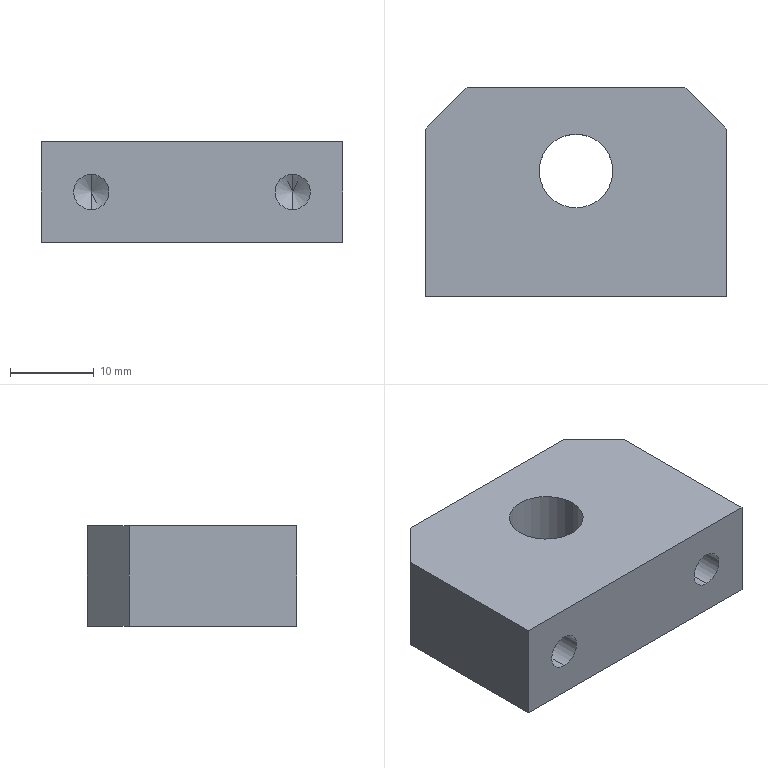Part | STEP file | 2037 Bag feed mounting plate 3 | 1 solid | 18 faces | box 36 x 25 x 12 mm | volume 9371 mm3 | plane 8 | cylinder 6 | cone 4 | commonest cylinder face diameters 4.2 x4 8.8 x2
STEP:
#1=CARTESIAN_POINT('',(0.,0.,0.));
#2=DIRECTION('',(0.,0.,1.));
#3=DIRECTION('',(1.,0.,0.));
#4=AXIS2_PLACEMENT_3D('',#1,#2,#3);
#5=CARTESIAN_POINT('',(12.,1.5,3.9));
#6=VERTEX_POINT('',#5);
#7=CARTESIAN_POINT('',(12.,-12.5,3.9));
#8=VERTEX_POINT('',#7);
#9=CARTESIAN_POINT('',(12.,-12.5,3.9));
#10=DIRECTION('',(0.,-1.,0.));
#11=VECTOR('',#10,1.);
#12=LINE('',#9,#11);
#13=CARTESIAN_POINT('',(12.,-12.5,6.));
#14=DIRECTION('',(0.,-1.,0.));
#15=DIRECTION('',(0.,0.,-1.));
#16=AXIS2_PLACEMENT_3D('',#13,#14,#15);
#17=CYLINDRICAL_SURFACE('',#16,2.1);
#18=CARTESIAN_POINT('',(6.283,0.));
#19=DIRECTION('',(0.,1.));
#20=VECTOR('',#19,1.);
#21=LINE('',#18,#20);
#22=(GEOMETRIC_REPRESENTATION_CONTEXT(2)PARAMETRIC_REPRESENTATION_CONTEXT()REPRESENTATION_CONTEXT('',''));
#23=DEFINITIONAL_REPRESENTATION('',(#21),#22);
#24=PCURVE('',#17,#23);
#25=CARTESIAN_POINT('',(12.,-12.5,6.));
#26=DIRECTION('',(0.,-1.,0.));
#27=DIRECTION('',(0.,0.,-1.));
#28=AXIS2_PLACEMENT_3D('',#25,#26,#27);
#29=CYLINDRICAL_SURFACE('',#28,2.1);
#30=CARTESIAN_POINT('',(0.,0.));
#31=DIRECTION('',(0.,1.));
#32=VECTOR('',#31,1.);
#33=LINE('',#30,#32);
#34=(GEOMETRIC_REPRESENTATION_CONTEXT(2)PARAMETRIC_REPRESENTATION_CONTEXT()REPRESENTATION_CONTEXT('',''));
#35=DEFINITIONAL_REPRESENTATION('',(#33),#34);
#36=PCURVE('',#29,#35);
#37=SURFACE_CURVE('',#12,(#24,#36),.PCURVE_S1.);
#38=EDGE_CURVE('',#6,#8,#37,.T.);
#39=ORIENTED_EDGE('',*,*,#38,.T.);
#40=CARTESIAN_POINT('',(12.,-12.5,8.1));
#41=VERTEX_POINT('',#40);
#42=CARTESIAN_POINT('',(12.,-12.5,6.));
#43=DIRECTION('',(0.,-1.,0.));
#44=DIRECTION('',(0.,0.,-1.));
#45=AXIS2_PLACEMENT_3D('',#42,#43,#44);
#46=CIRCLE('',#45,2.1);
#47=CARTESIAN_POINT('',(0.,0.));
#48=DIRECTION('',(1.,0.));
#49=VECTOR('',#48,1.);
#50=LINE('',#47,#49);
#51=(GEOMETRIC_REPRESENTATION_CONTEXT(2)PARAMETRIC_REPRESENTATION_CONTEXT()REPRESENTATION_CONTEXT('',''));
#52=DEFINITIONAL_REPRESENTATION('',(#50),#51);
#53=PCURVE('',#17,#52);
#54=CARTESIAN_POINT('',(-18.,-12.5,12.));
#55=DIRECTION('',(0.,1.,0.));
#56=DIRECTION('',(0.,0.,1.));
#57=AXIS2_PLACEMENT_3D('',#54,#55,#56);
#58=PLANE('',#57);
#59=CARTESIAN_POINT('',(-8.1,30.));
#60=CARTESIAN_POINT('',(-8.1,33.637));
#61=CARTESIAN_POINT('',(-4.95,31.819));
#62=CARTESIAN_POINT('',(-1.8,30.));
#63=CARTESIAN_POINT('',(-4.95,28.181));
#64=CARTESIAN_POINT('',(-8.1,26.363));
#65=CARTESIAN_POINT('',(-8.1,30.));
#66=(BOUNDED_CURVE()B_SPLINE_CURVE(2,(#59,#60,#61,#62,#63,#64,#65),.UNSPECIFIED.,.T.,.F.)B_SPLINE_CURVE_WITH_KNOTS((1,2,2,2,2,1),(-2.094,0.,2.094,4.189,6.283,8.378),.UNSPECIFIED.)CURVE()GEOMETRIC_REPRESENTATION_ITEM()RATIONAL_B_SPLINE_CURVE((1.,0.5,1.,0.5,1.,0.5,1.))REPRESENTATION_ITEM(''));
#67=(GEOMETRIC_REPRESENTATION_CONTEXT(2)PARAMETRIC_REPRESENTATION_CONTEXT()REPRESENTATION_CONTEXT('',''));
#68=DEFINITIONAL_REPRESENTATION('',(#66),#67);
#69=PCURVE('',#58,#68);
#70=SURFACE_CURVE('',#46,(#53,#69),.PCURVE_S1.);
#71=EDGE_CURVE('',#41,#8,#70,.T.);
#72=ORIENTED_EDGE('',*,*,#71,.F.);
#73=CARTESIAN_POINT('',(12.,1.5,8.1));
#74=VERTEX_POINT('',#73);
#75=CARTESIAN_POINT('',(12.,-12.5,8.1));
#76=DIRECTION('',(0.,-1.,0.));
#77=VECTOR('',#76,1.);
#78=LINE('',#75,#77);
#79=CARTESIAN_POINT('',(3.142,0.));
#80=DIRECTION('',(0.,1.));
#81=VECTOR('',#80,1.);
#82=LINE('',#79,#81);
#83=(GEOMETRIC_REPRESENTATION_CONTEXT(2)PARAMETRIC_REPRESENTATION_CONTEXT()REPRESENTATION_CONTEXT('',''));
#84=DEFINITIONAL_REPRESENTATION('',(#82),#83);
#85=PCURVE('',#17,#84);
#86=CARTESIAN_POINT('',(3.142,0.));
#87=DIRECTION('',(0.,1.));
#88=VECTOR('',#87,1.);
#89=LINE('',#86,#88);
#90=(GEOMETRIC_REPRESENTATION_CONTEXT(2)PARAMETRIC_REPRESENTATION_CONTEXT()REPRESENTATION_CONTEXT('',''));
#91=DEFINITIONAL_REPRESENTATION('',(#89),#90);
#92=PCURVE('',#29,#91);
#93=SURFACE_CURVE('',#78,(#85,#92),.PCURVE_S1.);
#94=EDGE_CURVE('',#74,#41,#93,.T.);
#95=ORIENTED_EDGE('',*,*,#94,.F.);
#96=CARTESIAN_POINT('',(12.,1.5,6.));
#97=DIRECTION('',(0.,-1.,0.));
#98=DIRECTION('',(0.,0.,-1.));
#99=AXIS2_PLACEMENT_3D('',#96,#97,#98);
#100=CIRCLE('',#99,2.1);
#101=CARTESIAN_POINT('',(0.,-14.));
#102=DIRECTION('',(1.,0.));
#103=VECTOR('',#102,1.);
#104=LINE('',#101,#103);
#105=(GEOMETRIC_REPRESENTATION_CONTEXT(2)PARAMETRIC_REPRESENTATION_CONTEXT()REPRESENTATION_CONTEXT('',''));
#106=DEFINITIONAL_REPRESENTATION('',(#104),#105);
#107=PCURVE('',#17,#106);
#108=CARTESIAN_POINT('',(12.,1.5,6.));
#109=DIRECTION('',(0.,-1.,0.));
#110=DIRECTION('',(0.,0.,-1.));
#111=AXIS2_PLACEMENT_3D('',#108,#109,#110);
#112=CONICAL_SURFACE('',#111,2.1,1.03);
#113=CARTESIAN_POINT('',(0.,0.));
#114=DIRECTION('',(1.,0.));
#115=VECTOR('',#114,1.);
#116=LINE('',#113,#115);
#117=(GEOMETRIC_REPRESENTATION_CONTEXT(2)PARAMETRIC_REPRESENTATION_CONTEXT()REPRESENTATION_CONTEXT('',''));
#118=DEFINITIONAL_REPRESENTATION('',(#116),#117);
#119=PCURVE('',#112,#118);
#120=SURFACE_CURVE('',#100,(#107,#119),.PCURVE_S1.);
#121=EDGE_CURVE('',#74,#6,#120,.T.);
#122=ORIENTED_EDGE('',*,*,#121,.T.);
#123=EDGE_LOOP('',(#39,#72,#95,#122));
#124=FACE_BOUND('',#123,.F.);
#125=ADVANCED_FACE('',(#124),#17,.F.);
#126=ORIENTED_EDGE('',*,*,#121,.F.);
#127=CARTESIAN_POINT('',(12.,2.762,6.));
#128=VERTEX_POINT('',#127);
#129=CARTESIAN_POINT('',(12.,1.5,8.1));
#130=DIRECTION('',(0.,-0.515,0.8572));
#131=VECTOR('',#130,1.);
#132=LINE('',#129,#131);
#133=CARTESIAN_POINT('',(3.142,0.));
#134=DIRECTION('',(0.,1.));
#135=VECTOR('',#134,1.);
#136=LINE('',#133,#135);
#137=(GEOMETRIC_REPRESENTATION_CONTEXT(2)PARAMETRIC_REPRESENTATION_CONTEXT()REPRESENTATION_CONTEXT('',''));
#138=DEFINITIONAL_REPRESENTATION('',(#136),#137);
#139=PCURVE('',#112,#138);
#140=CARTESIAN_POINT('',(12.,1.5,6.));
#141=DIRECTION('',(0.,-1.,0.));
#142=DIRECTION('',(0.,0.,-1.));
#143=AXIS2_PLACEMENT_3D('',#140,#141,#142);
#144=CONICAL_SURFACE('',#143,2.1,1.03);
#145=CARTESIAN_POINT('',(3.142,0.));
#146=DIRECTION('',(0.,1.));
#147=VECTOR('',#146,1.);
#148=LINE('',#145,#147);
#149=(GEOMETRIC_REPRESENTATION_CONTEXT(2)PARAMETRIC_REPRESENTATION_CONTEXT()REPRESENTATION_CONTEXT('',''));
#150=DEFINITIONAL_REPRESENTATION('',(#148),#149);
#151=PCURVE('',#144,#150);
#152=SURFACE_CURVE('',#132,(#139,#151),.PCURVE_S1.);
#153=EDGE_CURVE('',#128,#74,#152,.T.);
#154=ORIENTED_EDGE('',*,*,#153,.F.);
#155=CARTESIAN_POINT('',(12.,1.5,3.9));
#156=DIRECTION('',(0.,-0.515,-0.8572));
#157=VECTOR('',#156,1.);
#158=LINE('',#155,#157);
#159=CARTESIAN_POINT('',(6.283,0.));
#160=DIRECTION('',(0.,1.));
#161=VECTOR('',#160,1.);
#162=LINE('',#159,#161);
#163=(GEOMETRIC_REPRESENTATION_CONTEXT(2)PARAMETRIC_REPRESENTATION_CONTEXT()REPRESENTATION_CONTEXT('',''));
#164=DEFINITIONAL_REPRESENTATION('',(#162),#163);
#165=PCURVE('',#112,#164);
#166=CARTESIAN_POINT('',(0.,0.));
#167=DIRECTION('',(0.,1.));
#168=VECTOR('',#167,1.);
#169=LINE('',#166,#168);
#170=(GEOMETRIC_REPRESENTATION_CONTEXT(2)PARAMETRIC_REPRESENTATION_CONTEXT()REPRESENTATION_CONTEXT('',''));
#171=DEFINITIONAL_REPRESENTATION('',(#169),#170);
#172=PCURVE('',#144,#171);
#173=SURFACE_CURVE('',#158,(#165,#172),.PCURVE_S1.);
#174=EDGE_CURVE('',#128,#6,#173,.T.);
#175=ORIENTED_EDGE('',*,*,#174,.T.);
#176=EDGE_LOOP('',(#126,#154,#175));
#177=FACE_BOUND('',#176,.F.);
#178=ADVANCED_FACE('',(#177),#112,.F.);
#179=CARTESIAN_POINT('',(-12.,1.5,3.9));
#180=VERTEX_POINT('',#179);
#181=CARTESIAN_POINT('',(-12.,-12.5,3.9));
#182=VERTEX_POINT('',#181);
#183=CARTESIAN_POINT('',(-12.,-12.5,3.9));
#184=DIRECTION('',(0.,-1.,0.));
#185=VECTOR('',#184,1.);
#186=LINE('',#183,#185);
#187=CARTESIAN_POINT('',(-12.,-12.5,6.));
#188=DIRECTION('',(0.,-1.,0.));
#189=DIRECTION('',(0.,0.,-1.));
#190=AXIS2_PLACEMENT_3D('',#187,#188,#189);
#191=CYLINDRICAL_SURFACE('',#190,2.1);
#192=CARTESIAN_POINT('',(6.283,0.));
#193=DIRECTION('',(0.,1.));
#194=VECTOR('',#193,1.);
#195=LINE('',#192,#194);
#196=(GEOMETRIC_REPRESENTATION_CONTEXT(2)PARAMETRIC_REPRESENTATION_CONTEXT()REPRESENTATION_CONTEXT('',''));
#197=DEFINITIONAL_REPRESENTATION('',(#195),#196);
#198=PCURVE('',#191,#197);
#199=CARTESIAN_POINT('',(-12.,-12.5,6.));
#200=DIRECTION('',(0.,-1.,0.));
#201=DIRECTION('',(0.,0.,-1.));
#202=AXIS2_PLACEMENT_3D('',#199,#200,#201);
#203=CYLINDRICAL_SURFACE('',#202,2.1);
#204=CARTESIAN_POINT('',(0.,0.));
#205=DIRECTION('',(0.,1.));
#206=VECTOR('',#205,1.);
#207=LINE('',#204,#206);
#208=(GEOMETRIC_REPRESENTATION_CONTEXT(2)PARAMETRIC_REPRESENTATION_CONTEXT()REPRESENTATION_CONTEXT('',''));
#209=DEFINITIONAL_REPRESENTATION('',(#207),#208);
#210=PCURVE('',#203,#209);
#211=SURFACE_CURVE('',#186,(#198,#210),.PCURVE_S1.);
#212=EDGE_CURVE('',#180,#182,#211,.T.);
#213=ORIENTED_EDGE('',*,*,#212,.T.);
#214=CARTESIAN_POINT('',(-12.,-12.5,8.1));
#215=VERTEX_POINT('',#214);
#216=CARTESIAN_POINT('',(-12.,-12.5,6.));
#217=DIRECTION('',(0.,-1.,0.));
#218=DIRECTION('',(0.,0.,-1.));
#219=AXIS2_PLACEMENT_3D('',#216,#217,#218);
#220=CIRCLE('',#219,2.1);
#221=CARTESIAN_POINT('',(0.,0.));
#222=DIRECTION('',(1.,0.));
#223=VECTOR('',#222,1.);
#224=LINE('',#221,#223);
#225=(GEOMETRIC_REPRESENTATION_CONTEXT(2)PARAMETRIC_REPRESENTATION_CONTEXT()REPRESENTATION_CONTEXT('',''));
#226=DEFINITIONAL_REPRESENTATION('',(#224),#225);
#227=PCURVE('',#191,#226);
#228=CARTESIAN_POINT('',(-8.1,6.));
#229=CARTESIAN_POINT('',(-8.1,9.637));
#230=CARTESIAN_POINT('',(-4.95,7.819));
#231=CARTESIAN_POINT('',(-1.8,6.));
#232=CARTESIAN_POINT('',(-4.95,4.181));
#233=CARTESIAN_POINT('',(-8.1,2.363));
#234=CARTESIAN_POINT('',(-8.1,6.));
#235=(BOUNDED_CURVE()B_SPLINE_CURVE(2,(#228,#229,#230,#231,#232,#233,#234),.UNSPECIFIED.,.T.,.F.)B_SPLINE_CURVE_WITH_KNOTS((1,2,2,2,2,1),(-2.094,0.,2.094,4.189,6.283,8.378),.UNSPECIFIED.)CURVE()GEOMETRIC_REPRESENTATION_ITEM()RATIONAL_B_SPLINE_CURVE((1.,0.5,1.,0.5,1.,0.5,1.))REPRESENTATION_ITEM(''));
#236=(GEOMETRIC_REPRESENTATION_CONTEXT(2)PARAMETRIC_REPRESENTATION_CONTEXT()REPRESENTATION_CONTEXT('',''));
#237=DEFINITIONAL_REPRESENTATION('',(#235),#236);
#238=PCURVE('',#58,#237);
#239=SURFACE_CURVE('',#220,(#227,#238),.PCURVE_S1.);
#240=EDGE_CURVE('',#215,#182,#239,.T.);
#241=ORIENTED_EDGE('',*,*,#240,.F.);
#242=CARTESIAN_POINT('',(-12.,1.5,8.1));
#243=VERTEX_POINT('',#242);
#244=CARTESIAN_POINT('',(-12.,-12.5,8.1));
#245=DIRECTION('',(0.,-1.,0.));
#246=VECTOR('',#245,1.);
#247=LINE('',#244,#246);
#248=CARTESIAN_POINT('',(3.142,0.));
#249=DIRECTION('',(0.,1.));
#250=VECTOR('',#249,1.);
#251=LINE('',#248,#250);
#252=(GEOMETRIC_REPRESENTATION_CONTEXT(2)PARAMETRIC_REPRESENTATION_CONTEXT()REPRESENTATION_CONTEXT('',''));
#253=DEFINITIONAL_REPRESENTATION('',(#251),#252);
#254=PCURVE('',#191,#253);
#255=CARTESIAN_POINT('',(3.142,0.));
#256=DIRECTION('',(0.,1.));
#257=VECTOR('',#256,1.);
#258=LINE('',#255,#257);
#259=(GEOMETRIC_REPRESENTATION_CONTEXT(2)PARAMETRIC_REPRESENTATION_CONTEXT()REPRESENTATION_CONTEXT('',''));
#260=DEFINITIONAL_REPRESENTATION('',(#258),#259);
#261=PCURVE('',#203,#260);
#262=SURFACE_CURVE('',#247,(#254,#261),.PCURVE_S1.);
#263=EDGE_CURVE('',#243,#215,#262,.T.);
#264=ORIENTED_EDGE('',*,*,#263,.F.);
#265=CARTESIAN_POINT('',(-12.,1.5,6.));
#266=DIRECTION('',(0.,-1.,0.));
#267=DIRECTION('',(0.,0.,-1.));
#268=AXIS2_PLACEMENT_3D('',#265,#266,#267);
#269=CIRCLE('',#268,2.1);
#270=CARTESIAN_POINT('',(0.,-14.));
#271=DIRECTION('',(1.,0.));
#272=VECTOR('',#271,1.);
#273=LINE('',#270,#272);
#274=(GEOMETRIC_REPRESENTATION_CONTEXT(2)PARAMETRIC_REPRESENTATION_CONTEXT()REPRESENTATION_CONTEXT('',''));
#275=DEFINITIONAL_REPRESENTATION('',(#273),#274);
#276=PCURVE('',#191,#275);
#277=CARTESIAN_POINT('',(-12.,1.5,6.));
#278=DIRECTION('',(0.,-1.,0.));
#279=DIRECTION('',(0.,0.,-1.));
#280=AXIS2_PLACEMENT_3D('',#277,#278,#279);
#281=CONICAL_SURFACE('',#280,2.1,1.03);
#282=CARTESIAN_POINT('',(0.,0.));
#283=DIRECTION('',(1.,0.));
#284=VECTOR('',#283,1.);
#285=LINE('',#282,#284);
#286=(GEOMETRIC_REPRESENTATION_CONTEXT(2)PARAMETRIC_REPRESENTATION_CONTEXT()REPRESENTATION_CONTEXT('',''));
#287=DEFINITIONAL_REPRESENTATION('',(#285),#286);
#288=PCURVE('',#281,#287);
#289=SURFACE_CURVE('',#269,(#276,#288),.PCURVE_S1.);
#290=EDGE_CURVE('',#243,#180,#289,.T.);
#291=ORIENTED_EDGE('',*,*,#290,.T.);
#292=EDGE_LOOP('',(#213,#241,#264,#291));
#293=FACE_BOUND('',#292,.F.);
#294=ADVANCED_FACE('',(#293),#191,.F.);
#295=ORIENTED_EDGE('',*,*,#290,.F.);
#296=CARTESIAN_POINT('',(-12.,2.762,6.));
#297=VERTEX_POINT('',#296);
#298=CARTESIAN_POINT('',(-12.,1.5,8.1));
#299=DIRECTION('',(0.,-0.515,0.8572));
#300=VECTOR('',#299,1.);
#301=LINE('',#298,#300);
#302=CARTESIAN_POINT('',(3.142,0.));
#303=DIRECTION('',(0.,1.));
#304=VECTOR('',#303,1.);
#305=LINE('',#302,#304);
#306=(GEOMETRIC_REPRESENTATION_CONTEXT(2)PARAMETRIC_REPRESENTATION_CONTEXT()REPRESENTATION_CONTEXT('',''));
#307=DEFINITIONAL_REPRESENTATION('',(#305),#306);
#308=PCURVE('',#281,#307);
#309=CARTESIAN_POINT('',(-12.,1.5,6.));
#310=DIRECTION('',(0.,-1.,0.));
#311=DIRECTION('',(0.,0.,-1.));
#312=AXIS2_PLACEMENT_3D('',#309,#310,#311);
#313=CONICAL_SURFACE('',#312,2.1,1.03);
#314=CARTESIAN_POINT('',(3.142,0.));
#315=DIRECTION('',(0.,1.));
#316=VECTOR('',#315,1.);
#317=LINE('',#314,#316);
#318=(GEOMETRIC_REPRESENTATION_CONTEXT(2)PARAMETRIC_REPRESENTATION_CONTEXT()REPRESENTATION_CONTEXT('',''));
#319=DEFINITIONAL_REPRESENTATION('',(#317),#318);
#320=PCURVE('',#313,#319);
#321=SURFACE_CURVE('',#301,(#308,#320),.PCURVE_S1.);
#322=EDGE_CURVE('',#297,#243,#321,.T.);
#323=ORIENTED_EDGE('',*,*,#322,.F.);
#324=CARTESIAN_POINT('',(-12.,1.5,3.9));
#325=DIRECTION('',(0.,-0.515,-0.8572));
#326=VECTOR('',#325,1.);
#327=LINE('',#324,#326);
#328=CARTESIAN_POINT('',(6.283,0.));
#329=DIRECTION('',(0.,1.));
#330=VECTOR('',#329,1.);
#331=LINE('',#328,#330);
#332=(GEOMETRIC_REPRESENTATION_CONTEXT(2)PARAMETRIC_REPRESENTATION_CONTEXT()REPRESENTATION_CONTEXT('',''));
#333=DEFINITIONAL_REPRESENTATION('',(#331),#332);
#334=PCURVE('',#281,#333);
#335=CARTESIAN_POINT('',(0.,0.));
#336=DIRECTION('',(0.,1.));
#337=VECTOR('',#336,1.);
#338=LINE('',#335,#337);
#339=(GEOMETRIC_REPRESENTATION_CONTEXT(2)PARAMETRIC_REPRESENTATION_CONTEXT()REPRESENTATION_CONTEXT('',''));
#340=DEFINITIONAL_REPRESENTATION('',(#338),#339);
#341=PCURVE('',#313,#340);
#342=SURFACE_CURVE('',#327,(#334,#341),.PCURVE_S1.);
#343=EDGE_CURVE('',#297,#180,#342,.T.);
#344=ORIENTED_EDGE('',*,*,#343,.T.);
#345=EDGE_LOOP('',(#295,#323,#344));
#346=FACE_BOUND('',#345,.F.);
#347=ADVANCED_FACE('',(#346),#281,.F.);
#348=CARTESIAN_POINT('',(4.4,2.5,0.));
#349=VERTEX_POINT('',#348);
#350=CARTESIAN_POINT('',(4.4,2.5,12.));
#351=VERTEX_POINT('',#350);
#352=CARTESIAN_POINT('',(4.4,2.5,12.));
#353=DIRECTION('',(0.,0.,1.));
#354=VECTOR('',#353,1.);
#355=LINE('',#352,#354);
#356=CARTESIAN_POINT('',(0.,2.5,12.));
#357=DIRECTION('',(0.,0.,1.));
#358=DIRECTION('',(1.,0.,0.));
#359=AXIS2_PLACEMENT_3D('',#356,#357,#358);
#360=CYLINDRICAL_SURFACE('',#359,4.4);
#361=CARTESIAN_POINT('',(6.283,0.));
#362=DIRECTION('',(0.,1.));
#363=VECTOR('',#362,1.);
#364=LINE('',#361,#363);
#365=(GEOMETRIC_REPRESENTATION_CONTEXT(2)PARAMETRIC_REPRESENTATION_CONTEXT()REPRESENTATION_CONTEXT('',''));
#366=DEFINITIONAL_REPRESENTATION('',(#364),#365);
#367=PCURVE('',#360,#366);
#368=CARTESIAN_POINT('',(0.,2.5,12.));
#369=DIRECTION('',(0.,0.,1.));
#370=DIRECTION('',(1.,0.,0.));
#371=AXIS2_PLACEMENT_3D('',#368,#369,#370);
#372=CYLINDRICAL_SURFACE('',#371,4.4);
#373=CARTESIAN_POINT('',(0.,0.));
#374=DIRECTION('',(0.,1.));
#375=VECTOR('',#374,1.);
#376=LINE('',#373,#375);
#377=(GEOMETRIC_REPRESENTATION_CONTEXT(2)PARAMETRIC_REPRESENTATION_CONTEXT()REPRESENTATION_CONTEXT('',''));
#378=DEFINITIONAL_REPRESENTATION('',(#376),#377);
#379=PCURVE('',#372,#378);
#380=SURFACE_CURVE('',#355,(#367,#379),.PCURVE_S1.);
#381=EDGE_CURVE('',#349,#351,#380,.T.);
#382=ORIENTED_EDGE('',*,*,#381,.T.);
#383=CARTESIAN_POINT('',(-4.4,2.5,12.));
#384=VERTEX_POINT('',#383);
#385=CARTESIAN_POINT('',(0.,2.5,12.));
#386=DIRECTION('',(0.,0.,1.));
#387=DIRECTION('',(1.,0.,0.));
#388=AXIS2_PLACEMENT_3D('',#385,#386,#387);
#389=CIRCLE('',#388,4.4);
#390=CARTESIAN_POINT('',(0.,0.));
#391=DIRECTION('',(1.,0.));
#392=VECTOR('',#391,1.);
#393=LINE('',#390,#392);
#394=(GEOMETRIC_REPRESENTATION_CONTEXT(2)PARAMETRIC_REPRESENTATION_CONTEXT()REPRESENTATION_CONTEXT('',''));
#395=DEFINITIONAL_REPRESENTATION('',(#393),#394);
#396=PCURVE('',#360,#395);
#397=CARTESIAN_POINT('',(0.,0.,12.));
#398=DIRECTION('',(0.,0.,-1.));
#399=DIRECTION('',(-1.,0.,0.));
#400=AXIS2_PLACEMENT_3D('',#397,#398,#399);
#401=PLANE('',#400);
#402=CARTESIAN_POINT('',(-4.4,2.5));
#403=CARTESIAN_POINT('',(-4.4,10.121));
#404=CARTESIAN_POINT('',(2.2,6.311));
#405=CARTESIAN_POINT('',(8.8,2.5));
#406=CARTESIAN_POINT('',(2.2,-1.311));
#407=CARTESIAN_POINT('',(-4.4,-5.121));
#408=CARTESIAN_POINT('',(-4.4,2.5));
#409=(BOUNDED_CURVE()B_SPLINE_CURVE(2,(#402,#403,#404,#405,#406,#407,#408),.UNSPECIFIED.,.T.,.F.)B_SPLINE_CURVE_WITH_KNOTS((1,2,2,2,2,1),(-2.094,0.,2.094,4.189,6.283,8.378),.UNSPECIFIED.)CURVE()GEOMETRIC_REPRESENTATION_ITEM()RATIONAL_B_SPLINE_CURVE((1.,0.5,1.,0.5,1.,0.5,1.))REPRESENTATION_ITEM(''));
#410=(GEOMETRIC_REPRESENTATION_CONTEXT(2)PARAMETRIC_REPRESENTATION_CONTEXT()REPRESENTATION_CONTEXT('',''));
#411=DEFINITIONAL_REPRESENTATION('',(#409),#410);
#412=PCURVE('',#401,#411);
#413=SURFACE_CURVE('',#389,(#396,#412),.PCURVE_S1.);
#414=EDGE_CURVE('',#384,#351,#413,.T.);
#415=ORIENTED_EDGE('',*,*,#414,.F.);
#416=CARTESIAN_POINT('',(-4.4,2.5,0.));
#417=VERTEX_POINT('',#416);
#418=CARTESIAN_POINT('',(-4.4,2.5,12.));
#419=DIRECTION('',(0.,0.,1.));
#420=VECTOR('',#419,1.);
#421=LINE('',#418,#420);
#422=CARTESIAN_POINT('',(3.142,0.));
#423=DIRECTION('',(0.,1.));
#424=VECTOR('',#423,1.);
#425=LINE('',#422,#424);
#426=(GEOMETRIC_REPRESENTATION_CONTEXT(2)PARAMETRIC_REPRESENTATION_CONTEXT()REPRESENTATION_CONTEXT('',''));
#427=DEFINITIONAL_REPRESENTATION('',(#425),#426);
#428=PCURVE('',#360,#427);
#429=CARTESIAN_POINT('',(3.142,0.));
#430=DIRECTION('',(0.,1.));
#431=VECTOR('',#430,1.);
#432=LINE('',#429,#431);
#433=(GEOMETRIC_REPRESENTATION_CONTEXT(2)PARAMETRIC_REPRESENTATION_CONTEXT()REPRESENTATION_CONTEXT('',''));
#434=DEFINITIONAL_REPRESENTATION('',(#432),#433);
#435=PCURVE('',#372,#434);
#436=SURFACE_CURVE('',#421,(#428,#435),.PCURVE_S1.);
#437=EDGE_CURVE('',#417,#384,#436,.T.);
#438=ORIENTED_EDGE('',*,*,#437,.F.);
#439=CARTESIAN_POINT('',(0.,2.5,0.));
#440=DIRECTION('',(0.,0.,1.));
#441=DIRECTION('',(1.,0.,0.));
#442=AXIS2_PLACEMENT_3D('',#439,#440,#441);
#443=CIRCLE('',#442,4.4);
#444=CARTESIAN_POINT('',(0.,-12.));
#445=DIRECTION('',(1.,0.));
#446=VECTOR('',#445,1.);
#447=LINE('',#444,#446);
#448=(GEOMETRIC_REPRESENTATION_CONTEXT(2)PARAMETRIC_REPRESENTATION_CONTEXT()REPRESENTATION_CONTEXT('',''));
#449=DEFINITIONAL_REPRESENTATION('',(#447),#448);
#450=PCURVE('',#360,#449);
#451=CARTESIAN_POINT('',(0.,0.,0.));
#452=DIRECTION('',(0.,0.,-1.));
#453=DIRECTION('',(-1.,0.,0.));
#454=AXIS2_PLACEMENT_3D('',#451,#452,#453);
#455=PLANE('',#454);
#456=CARTESIAN_POINT('',(-4.4,2.5));
#457=CARTESIAN_POINT('',(-4.4,10.121));
#458=CARTESIAN_POINT('',(2.2,6.311));
#459=CARTESIAN_POINT('',(8.8,2.5));
#460=CARTESIAN_POINT('',(2.2,-1.311));
#461=CARTESIAN_POINT('',(-4.4,-5.121));
#462=CARTESIAN_POINT('',(-4.4,2.5));
#463=(BOUNDED_CURVE()B_SPLINE_CURVE(2,(#456,#457,#458,#459,#460,#461,#462),.UNSPECIFIED.,.T.,.F.)B_SPLINE_CURVE_WITH_KNOTS((1,2,2,2,2,1),(-2.094,0.,2.094,4.189,6.283,8.378),.UNSPECIFIED.)CURVE()GEOMETRIC_REPRESENTATION_ITEM()RATIONAL_B_SPLINE_CURVE((1.,0.5,1.,0.5,1.,0.5,1.))REPRESENTATION_ITEM(''));
#464=(GEOMETRIC_REPRESENTATION_CONTEXT(2)PARAMETRIC_REPRESENTATION_CONTEXT()REPRESENTATION_CONTEXT('',''));
#465=DEFINITIONAL_REPRESENTATION('',(#463),#464);
#466=PCURVE('',#455,#465);
#467=SURFACE_CURVE('',#443,(#450,#466),.PCURVE_S1.);
#468=EDGE_CURVE('',#417,#349,#467,.T.);
#469=ORIENTED_EDGE('',*,*,#468,.T.);
#470=EDGE_LOOP('',(#382,#415,#438,#469));
#471=FACE_BOUND('',#470,.F.);
#472=ADVANCED_FACE('',(#471),#360,.F.);
#473=CARTESIAN_POINT('',(18.,-12.5,0.));
#474=VERTEX_POINT('',#473);
#475=CARTESIAN_POINT('',(18.,7.5,0.));
#476=VERTEX_POINT('',#475);
#477=CARTESIAN_POINT('',(18.,-12.5,0.));
#478=DIRECTION('',(0.,1.,0.));
#479=VECTOR('',#478,1.);
#480=LINE('',#477,#479);
#481=CARTESIAN_POINT('',(18.,-12.5,12.));
#482=DIRECTION('',(-1.,0.,0.));
#483=DIRECTION('',(0.,0.,1.));
#484=AXIS2_PLACEMENT_3D('',#481,#482,#483);
#485=PLANE('',#484);
#486=CARTESIAN_POINT('',(-12.,0.));
#487=DIRECTION('',(0.,1.));
#488=VECTOR('',#487,1.);
#489=LINE('',#486,#488);
#490=(GEOMETRIC_REPRESENTATION_CONTEXT(2)PARAMETRIC_REPRESENTATION_CONTEXT()REPRESENTATION_CONTEXT('',''));
#491=DEFINITIONAL_REPRESENTATION('',(#489),#490);
#492=PCURVE('',#485,#491);
#493=CARTESIAN_POINT('',(-18.,-12.5));
#494=DIRECTION('',(0.,1.));
#495=VECTOR('',#494,1.);
#496=LINE('',#493,#495);
#497=(GEOMETRIC_REPRESENTATION_CONTEXT(2)PARAMETRIC_REPRESENTATION_CONTEXT()REPRESENTATION_CONTEXT('',''));
#498=DEFINITIONAL_REPRESENTATION('',(#496),#497);
#499=PCURVE('',#455,#498);
#500=SURFACE_CURVE('',#480,(#492,#499),.PCURVE_S1.);
#501=EDGE_CURVE('',#474,#476,#500,.T.);
#502=ORIENTED_EDGE('',*,*,#501,.T.);
#503=CARTESIAN_POINT('',(18.,7.5,12.));
#504=VERTEX_POINT('',#503);
#505=CARTESIAN_POINT('',(18.,7.5,12.));
#506=DIRECTION('',(0.,0.,1.));
#507=VECTOR('',#506,1.);
#508=LINE('',#505,#507);
#509=CARTESIAN_POINT('',(0.,20.));
#510=DIRECTION('',(1.,0.));
#511=VECTOR('',#510,1.);
#512=LINE('',#509,#511);
#513=(GEOMETRIC_REPRESENTATION_CONTEXT(2)PARAMETRIC_REPRESENTATION_CONTEXT()REPRESENTATION_CONTEXT('',''));
#514=DEFINITIONAL_REPRESENTATION('',(#512),#513);
#515=PCURVE('',#485,#514);
#516=CARTESIAN_POINT('',(13.,12.5,12.));
#517=DIRECTION('',(-0.7071,-0.7071,0.));
#518=DIRECTION('',(0.,0.,-1.));
#519=AXIS2_PLACEMENT_3D('',#516,#517,#518);
#520=PLANE('',#519);
#521=CARTESIAN_POINT('',(0.,7.071));
#522=DIRECTION('',(-1.,0.));
#523=VECTOR('',#522,1.);
#524=LINE('',#521,#523);
#525=(GEOMETRIC_REPRESENTATION_CONTEXT(2)PARAMETRIC_REPRESENTATION_CONTEXT()REPRESENTATION_CONTEXT('',''));
#526=DEFINITIONAL_REPRESENTATION('',(#524),#525);
#527=PCURVE('',#520,#526);
#528=SURFACE_CURVE('',#508,(#515,#527),.PCURVE_S1.);
#529=EDGE_CURVE('',#476,#504,#528,.T.);
#530=ORIENTED_EDGE('',*,*,#529,.T.);
#531=CARTESIAN_POINT('',(18.,-12.5,12.));
#532=VERTEX_POINT('',#531);
#533=CARTESIAN_POINT('',(18.,-12.5,12.));
#534=DIRECTION('',(0.,1.,0.));
#535=VECTOR('',#534,1.);
#536=LINE('',#533,#535);
#537=CARTESIAN_POINT('',(0.,0.));
#538=DIRECTION('',(0.,1.));
#539=VECTOR('',#538,1.);
#540=LINE('',#537,#539);
#541=(GEOMETRIC_REPRESENTATION_CONTEXT(2)PARAMETRIC_REPRESENTATION_CONTEXT()REPRESENTATION_CONTEXT('',''));
#542=DEFINITIONAL_REPRESENTATION('',(#540),#541);
#543=PCURVE('',#485,#542);
#544=CARTESIAN_POINT('',(-18.,-12.5));
#545=DIRECTION('',(0.,1.));
#546=VECTOR('',#545,1.);
#547=LINE('',#544,#546);
#548=(GEOMETRIC_REPRESENTATION_CONTEXT(2)PARAMETRIC_REPRESENTATION_CONTEXT()REPRESENTATION_CONTEXT('',''));
#549=DEFINITIONAL_REPRESENTATION('',(#547),#548);
#550=PCURVE('',#401,#549);
#551=SURFACE_CURVE('',#536,(#543,#550),.PCURVE_S1.);
#552=EDGE_CURVE('',#532,#504,#551,.T.);
#553=ORIENTED_EDGE('',*,*,#552,.F.);
#554=CARTESIAN_POINT('',(18.,-12.5,12.));
#555=DIRECTION('',(0.,0.,-1.));
#556=VECTOR('',#555,1.);
#557=LINE('',#554,#556);
#558=CARTESIAN_POINT('',(0.,0.));
#559=DIRECTION('',(-1.,0.));
#560=VECTOR('',#559,1.);
#561=LINE('',#558,#560);
#562=(GEOMETRIC_REPRESENTATION_CONTEXT(2)PARAMETRIC_REPRESENTATION_CONTEXT()REPRESENTATION_CONTEXT('',''));
#563=DEFINITIONAL_REPRESENTATION('',(#561),#562);
#564=PCURVE('',#485,#563);
#565=CARTESIAN_POINT('',(0.,36.));
#566=DIRECTION('',(-1.,0.));
#567=VECTOR('',#566,1.);
#568=LINE('',#565,#567);
#569=(GEOMETRIC_REPRESENTATION_CONTEXT(2)PARAMETRIC_REPRESENTATION_CONTEXT()REPRESENTATION_CONTEXT('',''));
#570=DEFINITIONAL_REPRESENTATION('',(#568),#569);
#571=PCURVE('',#58,#570);
#572=SURFACE_CURVE('',#557,(#564,#571),.PCURVE_S1.);
#573=EDGE_CURVE('',#532,#474,#572,.T.);
#574=ORIENTED_EDGE('',*,*,#573,.T.);
#575=EDGE_LOOP('',(#502,#530,#553,#574));
#576=FACE_BOUND('',#575,.T.);
#577=ADVANCED_FACE('',(#576),#485,.F.);
#578=CARTESIAN_POINT('',(13.,12.5,12.));
#579=VERTEX_POINT('',#578);
#580=CARTESIAN_POINT('',(-13.,12.5,12.));
#581=VERTEX_POINT('',#580);
#582=CARTESIAN_POINT('',(-18.,12.5,12.));
#583=DIRECTION('',(-1.,0.,0.));
#584=VECTOR('',#583,1.);
#585=LINE('',#582,#584);
#586=CARTESIAN_POINT('',(-18.,12.5,12.));
#587=DIRECTION('',(0.,-1.,0.));
#588=DIRECTION('',(0.,0.,-1.));
#589=AXIS2_PLACEMENT_3D('',#586,#587,#588);
#590=PLANE('',#589);
#591=CARTESIAN_POINT('',(0.,0.));
#592=DIRECTION('',(0.,-1.));
#593=VECTOR('',#592,1.);
#594=LINE('',#591,#593);
#595=(GEOMETRIC_REPRESENTATION_CONTEXT(2)PARAMETRIC_REPRESENTATION_CONTEXT()REPRESENTATION_CONTEXT('',''));
#596=DEFINITIONAL_REPRESENTATION('',(#594),#595);
#597=PCURVE('',#590,#596);
#598=CARTESIAN_POINT('',(18.,12.5));
#599=DIRECTION('',(1.,0.));
#600=VECTOR('',#599,1.);
#601=LINE('',#598,#600);
#602=(GEOMETRIC_REPRESENTATION_CONTEXT(2)PARAMETRIC_REPRESENTATION_CONTEXT()REPRESENTATION_CONTEXT('',''));
#603=DEFINITIONAL_REPRESENTATION('',(#601),#602);
#604=PCURVE('',#401,#603);
#605=SURFACE_CURVE('',#585,(#597,#604),.PCURVE_S1.);
#606=EDGE_CURVE('',#579,#581,#605,.T.);
#607=ORIENTED_EDGE('',*,*,#606,.F.);
#608=CARTESIAN_POINT('',(13.,12.5,0.));
#609=VERTEX_POINT('',#608);
#610=CARTESIAN_POINT('',(13.,12.5,12.));
#611=DIRECTION('',(0.,0.,-1.));
#612=VECTOR('',#611,1.);
#613=LINE('',#610,#612);
#614=CARTESIAN_POINT('',(0.,31.));
#615=DIRECTION('',(1.,0.));
#616=VECTOR('',#615,1.);
#617=LINE('',#614,#616);
#618=(GEOMETRIC_REPRESENTATION_CONTEXT(2)PARAMETRIC_REPRESENTATION_CONTEXT()REPRESENTATION_CONTEXT('',''));
#619=DEFINITIONAL_REPRESENTATION('',(#617),#618);
#620=PCURVE('',#590,#619);
#621=CARTESIAN_POINT('',(0.,0.));
#622=DIRECTION('',(1.,0.));
#623=VECTOR('',#622,1.);
#624=LINE('',#621,#623);
#625=(GEOMETRIC_REPRESENTATION_CONTEXT(2)PARAMETRIC_REPRESENTATION_CONTEXT()REPRESENTATION_CONTEXT('',''));
#626=DEFINITIONAL_REPRESENTATION('',(#624),#625);
#627=PCURVE('',#520,#626);
#628=SURFACE_CURVE('',#613,(#620,#627),.PCURVE_S1.);
#629=EDGE_CURVE('',#579,#609,#628,.T.);
#630=ORIENTED_EDGE('',*,*,#629,.T.);
#631=CARTESIAN_POINT('',(-13.,12.5,0.));
#632=VERTEX_POINT('',#631);
#633=CARTESIAN_POINT('',(-18.,12.5,0.));
#634=DIRECTION('',(-1.,0.,0.));
#635=VECTOR('',#634,1.);
#636=LINE('',#633,#635);
#637=CARTESIAN_POINT('',(12.,0.));
#638=DIRECTION('',(0.,-1.));
#639=VECTOR('',#638,1.);
#640=LINE('',#637,#639);
#641=(GEOMETRIC_REPRESENTATION_CONTEXT(2)PARAMETRIC_REPRESENTATION_CONTEXT()REPRESENTATION_CONTEXT('',''));
#642=DEFINITIONAL_REPRESENTATION('',(#640),#641);
#643=PCURVE('',#590,#642);
#644=CARTESIAN_POINT('',(18.,12.5));
#645=DIRECTION('',(1.,0.));
#646=VECTOR('',#645,1.);
#647=LINE('',#644,#646);
#648=(GEOMETRIC_REPRESENTATION_CONTEXT(2)PARAMETRIC_REPRESENTATION_CONTEXT()REPRESENTATION_CONTEXT('',''));
#649=DEFINITIONAL_REPRESENTATION('',(#647),#648);
#650=PCURVE('',#455,#649);
#651=SURFACE_CURVE('',#636,(#643,#650),.PCURVE_S1.);
#652=EDGE_CURVE('',#609,#632,#651,.T.);
#653=ORIENTED_EDGE('',*,*,#652,.T.);
#654=CARTESIAN_POINT('',(-13.,12.5,12.));
#655=DIRECTION('',(0.,0.,1.));
#656=VECTOR('',#655,1.);
#657=LINE('',#654,#656);
#658=CARTESIAN_POINT('',(0.,5.));
#659=DIRECTION('',(-1.,0.));
#660=VECTOR('',#659,1.);
#661=LINE('',#658,#660);
#662=(GEOMETRIC_REPRESENTATION_CONTEXT(2)PARAMETRIC_REPRESENTATION_CONTEXT()REPRESENTATION_CONTEXT('',''));
#663=DEFINITIONAL_REPRESENTATION('',(#661),#662);
#664=PCURVE('',#590,#663);
#665=CARTESIAN_POINT('',(-18.,7.5,12.));
#666=DIRECTION('',(0.7071,-0.7071,0.));
#667=DIRECTION('',(0.,0.,-1.));
#668=AXIS2_PLACEMENT_3D('',#665,#666,#667);
#669=PLANE('',#668);
#670=CARTESIAN_POINT('',(0.,7.071));
#671=DIRECTION('',(-1.,0.));
#672=VECTOR('',#671,1.);
#673=LINE('',#670,#672);
#674=(GEOMETRIC_REPRESENTATION_CONTEXT(2)PARAMETRIC_REPRESENTATION_CONTEXT()REPRESENTATION_CONTEXT('',''));
#675=DEFINITIONAL_REPRESENTATION('',(#673),#674);
#676=PCURVE('',#669,#675);
#677=SURFACE_CURVE('',#657,(#664,#676),.PCURVE_S1.);
#678=EDGE_CURVE('',#632,#581,#677,.T.);
#679=ORIENTED_EDGE('',*,*,#678,.T.);
#680=EDGE_LOOP('',(#607,#630,#653,#679));
#681=FACE_BOUND('',#680,.T.);
#682=ADVANCED_FACE('',(#681),#590,.F.);
#683=CARTESIAN_POINT('',(-18.,7.5,12.));
#684=VERTEX_POINT('',#683);
#685=CARTESIAN_POINT('',(-18.,-12.5,12.));
#686=VERTEX_POINT('',#685);
#687=CARTESIAN_POINT('',(-18.,-12.5,12.));
#688=DIRECTION('',(0.,-1.,0.));
#689=VECTOR('',#688,1.);
#690=LINE('',#687,#689);
#691=CARTESIAN_POINT('',(-18.,-12.5,12.));
#692=DIRECTION('',(1.,0.,0.));
#693=DIRECTION('',(0.,0.,-1.));
#694=AXIS2_PLACEMENT_3D('',#691,#692,#693);
#695=PLANE('',#694);
#696=CARTESIAN_POINT('',(0.,0.));
#697=DIRECTION('',(0.,-1.));
#698=VECTOR('',#697,1.);
#699=LINE('',#696,#698);
#700=(GEOMETRIC_REPRESENTATION_CONTEXT(2)PARAMETRIC_REPRESENTATION_CONTEXT()REPRESENTATION_CONTEXT('',''));
#701=DEFINITIONAL_REPRESENTATION('',(#699),#700);
#702=PCURVE('',#695,#701);
#703=CARTESIAN_POINT('',(18.,-12.5));
#704=DIRECTION('',(0.,-1.));
#705=VECTOR('',#704,1.);
#706=LINE('',#703,#705);
#707=(GEOMETRIC_REPRESENTATION_CONTEXT(2)PARAMETRIC_REPRESENTATION_CONTEXT()REPRESENTATION_CONTEXT('',''));
#708=DEFINITIONAL_REPRESENTATION('',(#706),#707);
#709=PCURVE('',#401,#708);
#710=SURFACE_CURVE('',#690,(#702,#709),.PCURVE_S1.);
#711=EDGE_CURVE('',#684,#686,#710,.T.);
#712=ORIENTED_EDGE('',*,*,#711,.F.);
#713=CARTESIAN_POINT('',(-18.,7.5,0.));
#714=VERTEX_POINT('',#713);
#715=CARTESIAN_POINT('',(-18.,7.5,12.));
#716=DIRECTION('',(0.,0.,-1.));
#717=VECTOR('',#716,1.);
#718=LINE('',#715,#717);
#719=CARTESIAN_POINT('',(0.,20.));
#720=DIRECTION('',(1.,0.));
#721=VECTOR('',#720,1.);
#722=LINE('',#719,#721);
#723=(GEOMETRIC_REPRESENTATION_CONTEXT(2)PARAMETRIC_REPRESENTATION_CONTEXT()REPRESENTATION_CONTEXT('',''));
#724=DEFINITIONAL_REPRESENTATION('',(#722),#723);
#725=PCURVE('',#695,#724);
#726=CARTESIAN_POINT('',(0.,0.));
#727=DIRECTION('',(1.,0.));
#728=VECTOR('',#727,1.);
#729=LINE('',#726,#728);
#730=(GEOMETRIC_REPRESENTATION_CONTEXT(2)PARAMETRIC_REPRESENTATION_CONTEXT()REPRESENTATION_CONTEXT('',''));
#731=DEFINITIONAL_REPRESENTATION('',(#729),#730);
#732=PCURVE('',#669,#731);
#733=SURFACE_CURVE('',#718,(#725,#732),.PCURVE_S1.);
#734=EDGE_CURVE('',#684,#714,#733,.T.);
#735=ORIENTED_EDGE('',*,*,#734,.T.);
#736=CARTESIAN_POINT('',(-18.,-12.5,0.));
#737=VERTEX_POINT('',#736);
#738=CARTESIAN_POINT('',(-18.,-12.5,0.));
#739=DIRECTION('',(0.,-1.,0.));
#740=VECTOR('',#739,1.);
#741=LINE('',#738,#740);
#742=CARTESIAN_POINT('',(12.,0.));
#743=DIRECTION('',(0.,-1.));
#744=VECTOR('',#743,1.);
#745=LINE('',#742,#744);
#746=(GEOMETRIC_REPRESENTATION_CONTEXT(2)PARAMETRIC_REPRESENTATION_CONTEXT()REPRESENTATION_CONTEXT('',''));
#747=DEFINITIONAL_REPRESENTATION('',(#745),#746);
#748=PCURVE('',#695,#747);
#749=CARTESIAN_POINT('',(18.,-12.5));
#750=DIRECTION('',(0.,-1.));
#751=VECTOR('',#750,1.);
#752=LINE('',#749,#751);
#753=(GEOMETRIC_REPRESENTATION_CONTEXT(2)PARAMETRIC_REPRESENTATION_CONTEXT()REPRESENTATION_CONTEXT('',''));
#754=DEFINITIONAL_REPRESENTATION('',(#752),#753);
#755=PCURVE('',#455,#754);
#756=SURFACE_CURVE('',#741,(#748,#755),.PCURVE_S1.);
#757=EDGE_CURVE('',#714,#737,#756,.T.);
#758=ORIENTED_EDGE('',*,*,#757,.T.);
#759=CARTESIAN_POINT('',(-18.,-12.5,12.));
#760=DIRECTION('',(0.,0.,-1.));
#761=VECTOR('',#760,1.);
#762=LINE('',#759,#761);
#763=CARTESIAN_POINT('',(0.,0.));
#764=DIRECTION('',(1.,0.));
#765=VECTOR('',#764,1.);
#766=LINE('',#763,#765);
#767=(GEOMETRIC_REPRESENTATION_CONTEXT(2)PARAMETRIC_REPRESENTATION_CONTEXT()REPRESENTATION_CONTEXT('',''));
#768=DEFINITIONAL_REPRESENTATION('',(#766),#767);
#769=PCURVE('',#695,#768);
#770=CARTESIAN_POINT('',(0.,0.));
#771=DIRECTION('',(-1.,0.));
#772=VECTOR('',#771,1.);
#773=LINE('',#770,#772);
#774=(GEOMETRIC_REPRESENTATION_CONTEXT(2)PARAMETRIC_REPRESENTATION_CONTEXT()REPRESENTATION_CONTEXT('',''));
#775=DEFINITIONAL_REPRESENTATION('',(#773),#774);
#776=PCURVE('',#58,#775);
#777=SURFACE_CURVE('',#762,(#769,#776),.PCURVE_S1.);
#778=EDGE_CURVE('',#686,#737,#777,.T.);
#779=ORIENTED_EDGE('',*,*,#778,.F.);
#780=EDGE_LOOP('',(#712,#735,#758,#779));
#781=FACE_BOUND('',#780,.T.);
#782=ADVANCED_FACE('',(#781),#695,.F.);
#783=CARTESIAN_POINT('',(12.,-12.5,6.));
#784=DIRECTION('',(0.,-1.,0.));
#785=DIRECTION('',(0.,0.,-1.));
#786=AXIS2_PLACEMENT_3D('',#783,#784,#785);
#787=CIRCLE('',#786,2.1);
#788=CARTESIAN_POINT('',(-8.1,30.));
#789=CARTESIAN_POINT('',(-8.1,33.637));
#790=CARTESIAN_POINT('',(-4.95,31.819));
#791=CARTESIAN_POINT('',(-1.8,30.));
#792=CARTESIAN_POINT('',(-4.95,28.181));
#793=CARTESIAN_POINT('',(-8.1,26.363));
#794=CARTESIAN_POINT('',(-8.1,30.));
#795=(BOUNDED_CURVE()B_SPLINE_CURVE(2,(#788,#789,#790,#791,#792,#793,#794),.UNSPECIFIED.,.T.,.F.)B_SPLINE_CURVE_WITH_KNOTS((1,2,2,2,2,1),(-2.094,0.,2.094,4.189,6.283,8.378),.UNSPECIFIED.)CURVE()GEOMETRIC_REPRESENTATION_ITEM()RATIONAL_B_SPLINE_CURVE((1.,0.5,1.,0.5,1.,0.5,1.))REPRESENTATION_ITEM(''));
#796=(GEOMETRIC_REPRESENTATION_CONTEXT(2)PARAMETRIC_REPRESENTATION_CONTEXT()REPRESENTATION_CONTEXT('',''));
#797=DEFINITIONAL_REPRESENTATION('',(#795),#796);
#798=PCURVE('',#58,#797);
#799=CARTESIAN_POINT('',(0.,0.));
#800=DIRECTION('',(1.,0.));
#801=VECTOR('',#800,1.);
#802=LINE('',#799,#801);
#803=(GEOMETRIC_REPRESENTATION_CONTEXT(2)PARAMETRIC_REPRESENTATION_CONTEXT()REPRESENTATION_CONTEXT('',''));
#804=DEFINITIONAL_REPRESENTATION('',(#802),#803);
#805=PCURVE('',#29,#804);
#806=SURFACE_CURVE('',#787,(#798,#805),.PCURVE_S1.);
#807=EDGE_CURVE('',#8,#41,#806,.T.);
#808=ORIENTED_EDGE('',*,*,#807,.F.);
#809=ORIENTED_EDGE('',*,*,#71,.F.);
#810=EDGE_LOOP('',(#808,#809));
#811=FACE_BOUND('',#810,.T.);
#812=CARTESIAN_POINT('',(-12.,-12.5,6.));
#813=DIRECTION('',(0.,-1.,0.));
#814=DIRECTION('',(0.,0.,-1.));
#815=AXIS2_PLACEMENT_3D('',#812,#813,#814);
#816=CIRCLE('',#815,2.1);
#817=CARTESIAN_POINT('',(-8.1,6.));
#818=CARTESIAN_POINT('',(-8.1,9.637));
#819=CARTESIAN_POINT('',(-4.95,7.819));
#820=CARTESIAN_POINT('',(-1.8,6.));
#821=CARTESIAN_POINT('',(-4.95,4.181));
#822=CARTESIAN_POINT('',(-8.1,2.363));
#823=CARTESIAN_POINT('',(-8.1,6.));
#824=(BOUNDED_CURVE()B_SPLINE_CURVE(2,(#817,#818,#819,#820,#821,#822,#823),.UNSPECIFIED.,.T.,.F.)B_SPLINE_CURVE_WITH_KNOTS((1,2,2,2,2,1),(-2.094,0.,2.094,4.189,6.283,8.378),.UNSPECIFIED.)CURVE()GEOMETRIC_REPRESENTATION_ITEM()RATIONAL_B_SPLINE_CURVE((1.,0.5,1.,0.5,1.,0.5,1.))REPRESENTATION_ITEM(''));
#825=(GEOMETRIC_REPRESENTATION_CONTEXT(2)PARAMETRIC_REPRESENTATION_CONTEXT()REPRESENTATION_CONTEXT('',''));
#826=DEFINITIONAL_REPRESENTATION('',(#824),#825);
#827=PCURVE('',#58,#826);
#828=CARTESIAN_POINT('',(0.,0.));
#829=DIRECTION('',(1.,0.));
#830=VECTOR('',#829,1.);
#831=LINE('',#828,#830);
#832=(GEOMETRIC_REPRESENTATION_CONTEXT(2)PARAMETRIC_REPRESENTATION_CONTEXT()REPRESENTATION_CONTEXT('',''));
#833=DEFINITIONAL_REPRESENTATION('',(#831),#832);
#834=PCURVE('',#203,#833);
#835=SURFACE_CURVE('',#816,(#827,#834),.PCURVE_S1.);
#836=EDGE_CURVE('',#182,#215,#835,.T.);
#837=ORIENTED_EDGE('',*,*,#836,.F.);
#838=ORIENTED_EDGE('',*,*,#240,.F.);
#839=EDGE_LOOP('',(#837,#838));
#840=FACE_BOUND('',#839,.T.);
#841=CARTESIAN_POINT('',(-18.,-12.5,0.));
#842=DIRECTION('',(1.,0.,0.));
#843=VECTOR('',#842,1.);
#844=LINE('',#841,#843);
#845=CARTESIAN_POINT('',(-12.,0.));
#846=DIRECTION('',(0.,1.));
#847=VECTOR('',#846,1.);
#848=LINE('',#845,#847);
#849=(GEOMETRIC_REPRESENTATION_CONTEXT(2)PARAMETRIC_REPRESENTATION_CONTEXT()REPRESENTATION_CONTEXT('',''));
#850=DEFINITIONAL_REPRESENTATION('',(#848),#849);
#851=PCURVE('',#58,#850);
#852=CARTESIAN_POINT('',(18.,-12.5));
#853=DIRECTION('',(-1.,0.));
#854=VECTOR('',#853,1.);
#855=LINE('',#852,#854);
#856=(GEOMETRIC_REPRESENTATION_CONTEXT(2)PARAMETRIC_REPRESENTATION_CONTEXT()REPRESENTATION_CONTEXT('',''));
#857=DEFINITIONAL_REPRESENTATION('',(#855),#856);
#858=PCURVE('',#455,#857);
#859=SURFACE_CURVE('',#844,(#851,#858),.PCURVE_S1.);
#860=EDGE_CURVE('',#737,#474,#859,.T.);
#861=ORIENTED_EDGE('',*,*,#860,.T.);
#862=ORIENTED_EDGE('',*,*,#573,.F.);
#863=CARTESIAN_POINT('',(-18.,-12.5,12.));
#864=DIRECTION('',(1.,0.,0.));
#865=VECTOR('',#864,1.);
#866=LINE('',#863,#865);
#867=CARTESIAN_POINT('',(0.,0.));
#868=DIRECTION('',(0.,1.));
#869=VECTOR('',#868,1.);
#870=LINE('',#867,#869);
#871=(GEOMETRIC_REPRESENTATION_CONTEXT(2)PARAMETRIC_REPRESENTATION_CONTEXT()REPRESENTATION_CONTEXT('',''));
#872=DEFINITIONAL_REPRESENTATION('',(#870),#871);
#873=PCURVE('',#58,#872);
#874=CARTESIAN_POINT('',(18.,-12.5));
#875=DIRECTION('',(-1.,0.));
#876=VECTOR('',#875,1.);
#877=LINE('',#874,#876);
#878=(GEOMETRIC_REPRESENTATION_CONTEXT(2)PARAMETRIC_REPRESENTATION_CONTEXT()REPRESENTATION_CONTEXT('',''));
#879=DEFINITIONAL_REPRESENTATION('',(#877),#878);
#880=PCURVE('',#401,#879);
#881=SURFACE_CURVE('',#866,(#873,#880),.PCURVE_S1.);
#882=EDGE_CURVE('',#686,#532,#881,.T.);
#883=ORIENTED_EDGE('',*,*,#882,.F.);
#884=ORIENTED_EDGE('',*,*,#778,.T.);
#885=EDGE_LOOP('',(#861,#862,#883,#884));
#886=FACE_BOUND('',#885,.T.);
#887=ADVANCED_FACE('',(#811,#840,#886),#58,.F.);
#888=CARTESIAN_POINT('',(0.,2.5,12.));
#889=DIRECTION('',(0.,0.,1.));
#890=DIRECTION('',(1.,0.,0.));
#891=AXIS2_PLACEMENT_3D('',#888,#889,#890);
#892=CIRCLE('',#891,4.4);
#893=CARTESIAN_POINT('',(-4.4,2.5));
#894=CARTESIAN_POINT('',(-4.4,10.121));
#895=CARTESIAN_POINT('',(2.2,6.311));
#896=CARTESIAN_POINT('',(8.8,2.5));
#897=CARTESIAN_POINT('',(2.2,-1.311));
#898=CARTESIAN_POINT('',(-4.4,-5.121));
#899=CARTESIAN_POINT('',(-4.4,2.5));
#900=(BOUNDED_CURVE()B_SPLINE_CURVE(2,(#893,#894,#895,#896,#897,#898,#899),.UNSPECIFIED.,.T.,.F.)B_SPLINE_CURVE_WITH_KNOTS((1,2,2,2,2,1),(-2.094,0.,2.094,4.189,6.283,8.378),.UNSPECIFIED.)CURVE()GEOMETRIC_REPRESENTATION_ITEM()RATIONAL_B_SPLINE_CURVE((1.,0.5,1.,0.5,1.,0.5,1.))REPRESENTATION_ITEM(''));
#901=(GEOMETRIC_REPRESENTATION_CONTEXT(2)PARAMETRIC_REPRESENTATION_CONTEXT()REPRESENTATION_CONTEXT('',''));
#902=DEFINITIONAL_REPRESENTATION('',(#900),#901);
#903=PCURVE('',#401,#902);
#904=CARTESIAN_POINT('',(0.,0.));
#905=DIRECTION('',(1.,0.));
#906=VECTOR('',#905,1.);
#907=LINE('',#904,#906);
#908=(GEOMETRIC_REPRESENTATION_CONTEXT(2)PARAMETRIC_REPRESENTATION_CONTEXT()REPRESENTATION_CONTEXT('',''));
#909=DEFINITIONAL_REPRESENTATION('',(#907),#908);
#910=PCURVE('',#372,#909);
#911=SURFACE_CURVE('',#892,(#903,#910),.PCURVE_S1.);
#912=EDGE_CURVE('',#351,#384,#911,.T.);
#913=ORIENTED_EDGE('',*,*,#912,.F.);
#914=ORIENTED_EDGE('',*,*,#414,.F.);
#915=EDGE_LOOP('',(#913,#914));
#916=FACE_BOUND('',#915,.T.);
#917=ORIENTED_EDGE('',*,*,#552,.T.);
#918=CARTESIAN_POINT('',(13.,12.5,12.));
#919=DIRECTION('',(-0.7071,0.7071,0.));
#920=VECTOR('',#919,1.);
#921=LINE('',#918,#920);
#922=CARTESIAN_POINT('',(-13.,12.5));
#923=DIRECTION('',(0.7071,0.7071));
#924=VECTOR('',#923,1.);
#925=LINE('',#922,#924);
#926=(GEOMETRIC_REPRESENTATION_CONTEXT(2)PARAMETRIC_REPRESENTATION_CONTEXT()REPRESENTATION_CONTEXT('',''));
#927=DEFINITIONAL_REPRESENTATION('',(#925),#926);
#928=PCURVE('',#401,#927);
#929=CARTESIAN_POINT('',(0.,0.));
#930=DIRECTION('',(0.,-1.));
#931=VECTOR('',#930,1.);
#932=LINE('',#929,#931);
#933=(GEOMETRIC_REPRESENTATION_CONTEXT(2)PARAMETRIC_REPRESENTATION_CONTEXT()REPRESENTATION_CONTEXT('',''));
#934=DEFINITIONAL_REPRESENTATION('',(#932),#933);
#935=PCURVE('',#520,#934);
#936=SURFACE_CURVE('',#921,(#928,#935),.PCURVE_S1.);
#937=EDGE_CURVE('',#504,#579,#936,.T.);
#938=ORIENTED_EDGE('',*,*,#937,.T.);
#939=ORIENTED_EDGE('',*,*,#606,.T.);
#940=CARTESIAN_POINT('',(-18.,7.5,12.));
#941=DIRECTION('',(-0.7071,-0.7071,0.));
#942=VECTOR('',#941,1.);
#943=LINE('',#940,#942);
#944=CARTESIAN_POINT('',(18.,7.5));
#945=DIRECTION('',(0.7071,-0.7071));
#946=VECTOR('',#945,1.);
#947=LINE('',#944,#946);
#948=(GEOMETRIC_REPRESENTATION_CONTEXT(2)PARAMETRIC_REPRESENTATION_CONTEXT()REPRESENTATION_CONTEXT('',''));
#949=DEFINITIONAL_REPRESENTATION('',(#947),#948);
#950=PCURVE('',#401,#949);
#951=CARTESIAN_POINT('',(0.,0.));
#952=DIRECTION('',(0.,-1.));
#953=VECTOR('',#952,1.);
#954=LINE('',#951,#953);
#955=(GEOMETRIC_REPRESENTATION_CONTEXT(2)PARAMETRIC_REPRESENTATION_CONTEXT()REPRESENTATION_CONTEXT('',''));
#956=DEFINITIONAL_REPRESENTATION('',(#954),#955);
#957=PCURVE('',#669,#956);
#958=SURFACE_CURVE('',#943,(#950,#957),.PCURVE_S1.);
#959=EDGE_CURVE('',#581,#684,#958,.T.);
#960=ORIENTED_EDGE('',*,*,#959,.T.);
#961=ORIENTED_EDGE('',*,*,#711,.T.);
#962=ORIENTED_EDGE('',*,*,#882,.T.);
#963=EDGE_LOOP('',(#917,#938,#939,#960,#961,#962));
#964=FACE_BOUND('',#963,.T.);
#965=ADVANCED_FACE('',(#916,#964),#401,.F.);
#966=CARTESIAN_POINT('',(0.,2.5,0.));
#967=DIRECTION('',(0.,0.,1.));
#968=DIRECTION('',(1.,0.,0.));
#969=AXIS2_PLACEMENT_3D('',#966,#967,#968);
#970=CIRCLE('',#969,4.4);
#971=CARTESIAN_POINT('',(-4.4,2.5));
#972=CARTESIAN_POINT('',(-4.4,10.121));
#973=CARTESIAN_POINT('',(2.2,6.311));
#974=CARTESIAN_POINT('',(8.8,2.5));
#975=CARTESIAN_POINT('',(2.2,-1.311));
#976=CARTESIAN_POINT('',(-4.4,-5.121));
#977=CARTESIAN_POINT('',(-4.4,2.5));
#978=(BOUNDED_CURVE()B_SPLINE_CURVE(2,(#971,#972,#973,#974,#975,#976,#977),.UNSPECIFIED.,.T.,.F.)B_SPLINE_CURVE_WITH_KNOTS((1,2,2,2,2,1),(-2.094,0.,2.094,4.189,6.283,8.378),.UNSPECIFIED.)CURVE()GEOMETRIC_REPRESENTATION_ITEM()RATIONAL_B_SPLINE_CURVE((1.,0.5,1.,0.5,1.,0.5,1.))REPRESENTATION_ITEM(''));
#979=(GEOMETRIC_REPRESENTATION_CONTEXT(2)PARAMETRIC_REPRESENTATION_CONTEXT()REPRESENTATION_CONTEXT('',''));
#980=DEFINITIONAL_REPRESENTATION('',(#978),#979);
#981=PCURVE('',#455,#980);
#982=CARTESIAN_POINT('',(0.,-12.));
#983=DIRECTION('',(1.,0.));
#984=VECTOR('',#983,1.);
#985=LINE('',#982,#984);
#986=(GEOMETRIC_REPRESENTATION_CONTEXT(2)PARAMETRIC_REPRESENTATION_CONTEXT()REPRESENTATION_CONTEXT('',''));
#987=DEFINITIONAL_REPRESENTATION('',(#985),#986);
#988=PCURVE('',#372,#987);
#989=SURFACE_CURVE('',#970,(#981,#988),.PCURVE_S1.);
#990=EDGE_CURVE('',#349,#417,#989,.T.);
#991=ORIENTED_EDGE('',*,*,#990,.T.);
#992=ORIENTED_EDGE('',*,*,#468,.T.);
#993=EDGE_LOOP('',(#991,#992));
#994=FACE_BOUND('',#993,.T.);
#995=ORIENTED_EDGE('',*,*,#652,.F.);
#996=CARTESIAN_POINT('',(12.75,12.75,0.));
#997=DIRECTION('',(0.7071,-0.7071,0.));
#998=VECTOR('',#997,1.);
#999=LINE('',#996,#998);
#1000=CARTESIAN_POINT('',(-12.75,12.75));
#1001=DIRECTION('',(-0.7071,-0.7071));
#1002=VECTOR('',#1001,1.);
#1003=LINE('',#1000,#1002);
#1004=(GEOMETRIC_REPRESENTATION_CONTEXT(2)PARAMETRIC_REPRESENTATION_CONTEXT()REPRESENTATION_CONTEXT('',''));
#1005=DEFINITIONAL_REPRESENTATION('',(#1003),#1004);
#1006=PCURVE('',#455,#1005);
#1007=CARTESIAN_POINT('',(12.,-0.3536));
#1008=DIRECTION('',(0.,1.));
#1009=VECTOR('',#1008,1.);
#1010=LINE('',#1007,#1009);
#1011=(GEOMETRIC_REPRESENTATION_CONTEXT(2)PARAMETRIC_REPRESENTATION_CONTEXT()REPRESENTATION_CONTEXT('',''));
#1012=DEFINITIONAL_REPRESENTATION('',(#1010),#1011);
#1013=PCURVE('',#520,#1012);
#1014=SURFACE_CURVE('',#999,(#1006,#1013),.PCURVE_S1.);
#1015=EDGE_CURVE('',#609,#476,#1014,.T.);
#1016=ORIENTED_EDGE('',*,*,#1015,.T.);
#1017=ORIENTED_EDGE('',*,*,#501,.F.);
#1018=ORIENTED_EDGE('',*,*,#860,.F.);
#1019=ORIENTED_EDGE('',*,*,#757,.F.);
#1020=CARTESIAN_POINT('',(-12.75,12.75,0.));
#1021=DIRECTION('',(0.7071,0.7071,0.));
#1022=VECTOR('',#1021,1.);
#1023=LINE('',#1020,#1022);
#1024=CARTESIAN_POINT('',(12.75,12.75));
#1025=DIRECTION('',(-0.7071,0.7071));
#1026=VECTOR('',#1025,1.);
#1027=LINE('',#1024,#1026);
#1028=(GEOMETRIC_REPRESENTATION_CONTEXT(2)PARAMETRIC_REPRESENTATION_CONTEXT()REPRESENTATION_CONTEXT('',''));
#1029=DEFINITIONAL_REPRESENTATION('',(#1027),#1028);
#1030=PCURVE('',#455,#1029);
#1031=CARTESIAN_POINT('',(12.,7.425));
#1032=DIRECTION('',(0.,1.));
#1033=VECTOR('',#1032,1.);
#1034=LINE('',#1031,#1033);
#1035=(GEOMETRIC_REPRESENTATION_CONTEXT(2)PARAMETRIC_REPRESENTATION_CONTEXT()REPRESENTATION_CONTEXT('',''));
#1036=DEFINITIONAL_REPRESENTATION('',(#1034),#1035);
#1037=PCURVE('',#669,#1036);
#1038=SURFACE_CURVE('',#1023,(#1030,#1037),.PCURVE_S1.);
#1039=EDGE_CURVE('',#714,#632,#1038,.T.);
#1040=ORIENTED_EDGE('',*,*,#1039,.T.);
#1041=EDGE_LOOP('',(#995,#1016,#1017,#1018,#1019,#1040));
#1042=FACE_BOUND('',#1041,.T.);
#1043=ADVANCED_FACE('',(#994,#1042),#455,.T.);
#1044=ORIENTED_EDGE('',*,*,#937,.F.);
#1045=ORIENTED_EDGE('',*,*,#529,.F.);
#1046=ORIENTED_EDGE('',*,*,#1015,.F.);
#1047=ORIENTED_EDGE('',*,*,#629,.F.);
#1048=EDGE_LOOP('',(#1044,#1045,#1046,#1047));
#1049=FACE_BOUND('',#1048,.T.);
#1050=ADVANCED_FACE('',(#1049),#520,.F.);
#1051=ORIENTED_EDGE('',*,*,#959,.F.);
#1052=ORIENTED_EDGE('',*,*,#678,.F.);
#1053=ORIENTED_EDGE('',*,*,#1039,.F.);
#1054=ORIENTED_EDGE('',*,*,#734,.F.);
#1055=EDGE_LOOP('',(#1051,#1052,#1053,#1054));
#1056=FACE_BOUND('',#1055,.T.);
#1057=ADVANCED_FACE('',(#1056),#669,.F.);
#1058=ORIENTED_EDGE('',*,*,#912,.F.);
#1059=ORIENTED_EDGE('',*,*,#381,.F.);
#1060=ORIENTED_EDGE('',*,*,#990,.T.);
#1061=ORIENTED_EDGE('',*,*,#437,.T.);
#1062=EDGE_LOOP('',(#1058,#1059,#1060,#1061));
#1063=FACE_BOUND('',#1062,.F.);
#1064=ADVANCED_FACE('',(#1063),#372,.F.);
#1065=CARTESIAN_POINT('',(-12.,1.5,6.));
#1066=DIRECTION('',(0.,-1.,0.));
#1067=DIRECTION('',(0.,0.,-1.));
#1068=AXIS2_PLACEMENT_3D('',#1065,#1066,#1067);
#1069=CIRCLE('',#1068,2.1);
#1070=CARTESIAN_POINT('',(0.,0.));
#1071=DIRECTION('',(1.,0.));
#1072=VECTOR('',#1071,1.);
#1073=LINE('',#1070,#1072);
#1074=(GEOMETRIC_REPRESENTATION_CONTEXT(2)PARAMETRIC_REPRESENTATION_CONTEXT()REPRESENTATION_CONTEXT('',''));
#1075=DEFINITIONAL_REPRESENTATION('',(#1073),#1074);
#1076=PCURVE('',#313,#1075);
#1077=CARTESIAN_POINT('',(0.,-14.));
#1078=DIRECTION('',(1.,0.));
#1079=VECTOR('',#1078,1.);
#1080=LINE('',#1077,#1079);
#1081=(GEOMETRIC_REPRESENTATION_CONTEXT(2)PARAMETRIC_REPRESENTATION_CONTEXT()REPRESENTATION_CONTEXT('',''));
#1082=DEFINITIONAL_REPRESENTATION('',(#1080),#1081);
#1083=PCURVE('',#203,#1082);
#1084=SURFACE_CURVE('',#1069,(#1076,#1083),.PCURVE_S1.);
#1085=EDGE_CURVE('',#180,#243,#1084,.T.);
#1086=ORIENTED_EDGE('',*,*,#1085,.F.);
#1087=ORIENTED_EDGE('',*,*,#343,.F.);
#1088=ORIENTED_EDGE('',*,*,#322,.T.);
#1089=EDGE_LOOP('',(#1086,#1087,#1088));
#1090=FACE_BOUND('',#1089,.F.);
#1091=ADVANCED_FACE('',(#1090),#313,.F.);
#1092=ORIENTED_EDGE('',*,*,#836,.F.);
#1093=ORIENTED_EDGE('',*,*,#212,.F.);
#1094=ORIENTED_EDGE('',*,*,#1085,.T.);
#1095=ORIENTED_EDGE('',*,*,#263,.T.);
#1096=EDGE_LOOP('',(#1092,#1093,#1094,#1095));
#1097=FACE_BOUND('',#1096,.F.);
#1098=ADVANCED_FACE('',(#1097),#203,.F.);
#1099=CARTESIAN_POINT('',(12.,1.5,6.));
#1100=DIRECTION('',(0.,-1.,0.));
#1101=DIRECTION('',(0.,0.,-1.));
#1102=AXIS2_PLACEMENT_3D('',#1099,#1100,#1101);
#1103=CIRCLE('',#1102,2.1);
#1104=CARTESIAN_POINT('',(0.,0.));
#1105=DIRECTION('',(1.,0.));
#1106=VECTOR('',#1105,1.);
#1107=LINE('',#1104,#1106);
#1108=(GEOMETRIC_REPRESENTATION_CONTEXT(2)PARAMETRIC_REPRESENTATION_CONTEXT()REPRESENTATION_CONTEXT('',''));
#1109=DEFINITIONAL_REPRESENTATION('',(#1107),#1108);
#1110=PCURVE('',#144,#1109);
#1111=CARTESIAN_POINT('',(0.,-14.));
#1112=DIRECTION('',(1.,0.));
#1113=VECTOR('',#1112,1.);
#1114=LINE('',#1111,#1113);
#1115=(GEOMETRIC_REPRESENTATION_CONTEXT(2)PARAMETRIC_REPRESENTATION_CONTEXT()REPRESENTATION_CONTEXT('',''));
#1116=DEFINITIONAL_REPRESENTATION('',(#1114),#1115);
#1117=PCURVE('',#29,#1116);
#1118=SURFACE_CURVE('',#1103,(#1110,#1117),.PCURVE_S1.);
#1119=EDGE_CURVE('',#6,#74,#1118,.T.);
#1120=ORIENTED_EDGE('',*,*,#1119,.F.);
#1121=ORIENTED_EDGE('',*,*,#174,.F.);
#1122=ORIENTED_EDGE('',*,*,#153,.T.);
#1123=EDGE_LOOP('',(#1120,#1121,#1122));
#1124=FACE_BOUND('',#1123,.F.);
#1125=ADVANCED_FACE('',(#1124),#144,.F.);
#1126=ORIENTED_EDGE('',*,*,#807,.F.);
#1127=ORIENTED_EDGE('',*,*,#38,.F.);
#1128=ORIENTED_EDGE('',*,*,#1119,.T.);
#1129=ORIENTED_EDGE('',*,*,#94,.T.);
#1130=EDGE_LOOP('',(#1126,#1127,#1128,#1129));
#1131=FACE_BOUND('',#1130,.F.);
#1132=ADVANCED_FACE('',(#1131),#29,.F.);
#1133=CLOSED_SHELL('',(#125,#178,#294,#347,#472,#577,#682,#782,#887,#965,#1043,#1050,#1057,#1064,#1091,#1098,#1125,#1132));
#1134=MANIFOLD_SOLID_BREP('',#1133);
#1135=(LENGTH_UNIT()NAMED_UNIT(*)SI_UNIT(.MILLI.,.METRE.));
#1136=UNCERTAINTY_MEASURE_WITH_UNIT(LENGTH_MEASURE(0.0000001),#1135,'','');
#1137=(NAMED_UNIT(*)PLANE_ANGLE_UNIT()SI_UNIT($,.RADIAN.));
#1138=(NAMED_UNIT(*)SI_UNIT($,.STERADIAN.)SOLID_ANGLE_UNIT());
#1139=(GEOMETRIC_REPRESENTATION_CONTEXT(3)GLOBAL_UNCERTAINTY_ASSIGNED_CONTEXT((#1136))GLOBAL_UNIT_ASSIGNED_CONTEXT((#1135,#1137,#1138))REPRESENTATION_CONTEXT('',''));
#1140=ADVANCED_BREP_SHAPE_REPRESENTATION('',(#4,#1134),#1139);